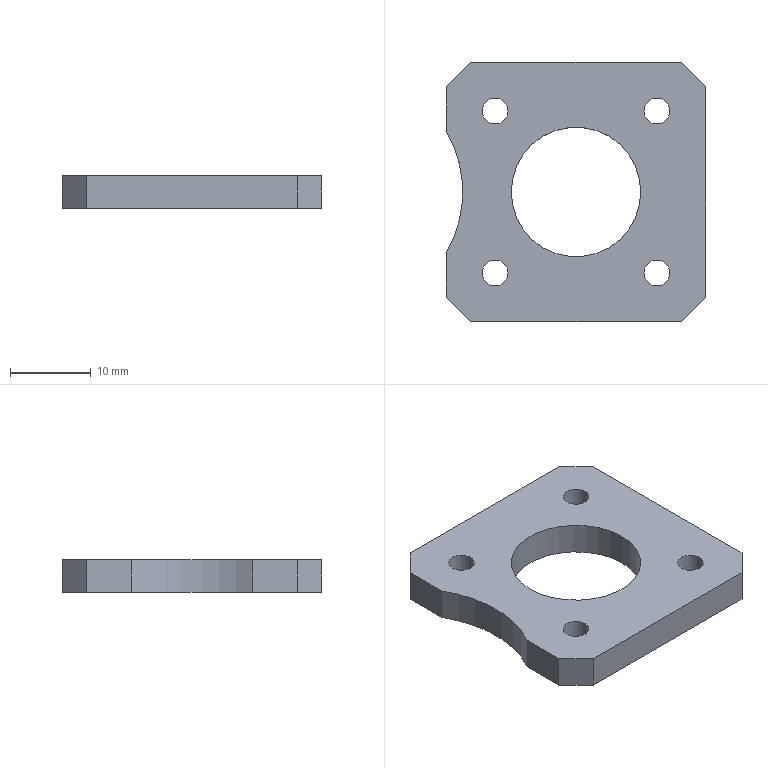Part | SolidWorks | features BaseBody 1 | 1 solid | 22 faces | box 32 x 32 x 4 mm | volume 3010 mm3 | cylinder 11 | plane 11 | commonest cylinder face diameters 3.2 x8 16 x2 30 x1
STEP:
#1=CARTESIAN_POINT('',(-11.6,10.,4.));
#2=VERTEX_POINT('',#1);
#3=CARTESIAN_POINT('',(-8.4,10.,4.));
#4=VERTEX_POINT('',#3);
#5=CARTESIAN_POINT('',(-10.,10.,4.));
#6=DIRECTION('',(0.,0.,1.));
#7=DIRECTION('',(-1.,0.,0.));
#8=AXIS2_PLACEMENT_3D('',#5,#6,#7);
#9=CIRCLE('',#8,1.6);
#10=EDGE_CURVE('',#2,#4,#9,.T.);
#11=ORIENTED_EDGE('',*,*,#10,.T.);
#12=CARTESIAN_POINT('',(-8.4,10.,0.));
#13=VERTEX_POINT('',#12);
#14=CARTESIAN_POINT('',(-8.4,10.,4.));
#15=DIRECTION('',(0.,0.,-1.));
#16=VECTOR('',#15,1000.);
#17=LINE('',#14,#16);
#18=EDGE_CURVE('',#4,#13,#17,.T.);
#19=ORIENTED_EDGE('',*,*,#18,.T.);
#20=CARTESIAN_POINT('',(-11.6,10.,0.));
#21=VERTEX_POINT('',#20);
#22=CARTESIAN_POINT('',(-10.,10.,0.));
#23=DIRECTION('',(0.,0.,-1.));
#24=DIRECTION('',(-1.,0.,0.));
#25=AXIS2_PLACEMENT_3D('',#22,#23,#24);
#26=CIRCLE('',#25,1.6);
#27=EDGE_CURVE('',#13,#21,#26,.T.);
#28=ORIENTED_EDGE('',*,*,#27,.T.);
#29=CARTESIAN_POINT('',(-11.6,10.,4.));
#30=DIRECTION('',(0.,0.,-1.));
#31=VECTOR('',#30,1000.);
#32=LINE('',#29,#31);
#33=EDGE_CURVE('',#2,#21,#32,.T.);
#34=ORIENTED_EDGE('',*,*,#33,.F.);
#35=EDGE_LOOP('',(#11,#19,#28,#34));
#36=FACE_OUTER_BOUND('',#35,.T.);
#37=CARTESIAN_POINT('',(-10.,10.,4.));
#38=DIRECTION('',(0.,0.,-1.));
#39=DIRECTION('',(-1.,0.,0.));
#40=AXIS2_PLACEMENT_3D('',#37,#38,#39);
#41=CYLINDRICAL_SURFACE('',#40,1.6);
#42=ADVANCED_FACE('',(#36),#41,.F.);
#43=CARTESIAN_POINT('',(8.,0.,4.));
#44=VERTEX_POINT('',#43);
#45=CARTESIAN_POINT('',(-8.,0.,4.));
#46=VERTEX_POINT('',#45);
#47=CARTESIAN_POINT('',(0.,0.,4.));
#48=DIRECTION('',(0.,0.,-1.));
#49=DIRECTION('',(-1.,0.,0.));
#50=AXIS2_PLACEMENT_3D('',#47,#48,#49);
#51=CIRCLE('',#50,8.);
#52=EDGE_CURVE('',#44,#46,#51,.T.);
#53=ORIENTED_EDGE('',*,*,#52,.F.);
#54=CARTESIAN_POINT('',(8.,0.,0.));
#55=VERTEX_POINT('',#54);
#56=CARTESIAN_POINT('',(8.,0.,4.));
#57=DIRECTION('',(0.,0.,-1.));
#58=VECTOR('',#57,1000.);
#59=LINE('',#56,#58);
#60=EDGE_CURVE('',#44,#55,#59,.T.);
#61=ORIENTED_EDGE('',*,*,#60,.T.);
#62=CARTESIAN_POINT('',(-8.,0.,0.));
#63=VERTEX_POINT('',#62);
#64=CARTESIAN_POINT('',(0.,0.,0.));
#65=DIRECTION('',(0.,0.,-1.));
#66=DIRECTION('',(-1.,0.,0.));
#67=AXIS2_PLACEMENT_3D('',#64,#65,#66);
#68=CIRCLE('',#67,8.);
#69=EDGE_CURVE('',#55,#63,#68,.T.);
#70=ORIENTED_EDGE('',*,*,#69,.T.);
#71=CARTESIAN_POINT('',(-8.,0.,4.));
#72=DIRECTION('',(0.,0.,-1.));
#73=VECTOR('',#72,1000.);
#74=LINE('',#71,#73);
#75=EDGE_CURVE('',#46,#63,#74,.T.);
#76=ORIENTED_EDGE('',*,*,#75,.F.);
#77=EDGE_LOOP('',(#53,#61,#70,#76));
#78=FACE_OUTER_BOUND('',#77,.T.);
#79=CARTESIAN_POINT('',(0.,0.,4.));
#80=DIRECTION('',(0.,0.,-1.));
#81=DIRECTION('',(-1.,0.,0.));
#82=AXIS2_PLACEMENT_3D('',#79,#80,#81);
#83=CYLINDRICAL_SURFACE('',#82,8.);
#84=ADVANCED_FACE('',(#78),#83,.F.);
#85=CARTESIAN_POINT('',(-8.4,-10.,4.));
#86=VERTEX_POINT('',#85);
#87=CARTESIAN_POINT('',(-11.6,-10.,4.));
#88=VERTEX_POINT('',#87);
#89=CARTESIAN_POINT('',(-10.,-10.,4.));
#90=DIRECTION('',(0.,0.,-1.));
#91=DIRECTION('',(-1.,0.,0.));
#92=AXIS2_PLACEMENT_3D('',#89,#90,#91);
#93=CIRCLE('',#92,1.6);
#94=EDGE_CURVE('',#86,#88,#93,.T.);
#95=ORIENTED_EDGE('',*,*,#94,.F.);
#96=CARTESIAN_POINT('',(-8.4,-10.,0.));
#97=VERTEX_POINT('',#96);
#98=CARTESIAN_POINT('',(-8.4,-10.,4.));
#99=DIRECTION('',(0.,0.,-1.));
#100=VECTOR('',#99,1000.);
#101=LINE('',#98,#100);
#102=EDGE_CURVE('',#86,#97,#101,.T.);
#103=ORIENTED_EDGE('',*,*,#102,.T.);
#104=CARTESIAN_POINT('',(-11.6,-10.,0.));
#105=VERTEX_POINT('',#104);
#106=CARTESIAN_POINT('',(-10.,-10.,0.));
#107=DIRECTION('',(0.,0.,-1.));
#108=DIRECTION('',(-1.,0.,0.));
#109=AXIS2_PLACEMENT_3D('',#106,#107,#108);
#110=CIRCLE('',#109,1.6);
#111=EDGE_CURVE('',#97,#105,#110,.T.);
#112=ORIENTED_EDGE('',*,*,#111,.T.);
#113=CARTESIAN_POINT('',(-11.6,-10.,4.));
#114=DIRECTION('',(0.,0.,-1.));
#115=VECTOR('',#114,1000.);
#116=LINE('',#113,#115);
#117=EDGE_CURVE('',#88,#105,#116,.T.);
#118=ORIENTED_EDGE('',*,*,#117,.F.);
#119=EDGE_LOOP('',(#95,#103,#112,#118));
#120=FACE_OUTER_BOUND('',#119,.T.);
#121=CARTESIAN_POINT('',(-10.,-10.,4.));
#122=DIRECTION('',(0.,0.,-1.));
#123=DIRECTION('',(-1.,0.,0.));
#124=AXIS2_PLACEMENT_3D('',#121,#122,#123);
#125=CYLINDRICAL_SURFACE('',#124,1.6);
#126=ADVANCED_FACE('',(#120),#125,.F.);
#127=CARTESIAN_POINT('',(11.6,-10.,4.));
#128=VERTEX_POINT('',#127);
#129=CARTESIAN_POINT('',(8.4,-10.,4.));
#130=VERTEX_POINT('',#129);
#131=CARTESIAN_POINT('',(10.,-10.,4.));
#132=DIRECTION('',(0.,0.,-1.));
#133=DIRECTION('',(-1.,0.,0.));
#134=AXIS2_PLACEMENT_3D('',#131,#132,#133);
#135=CIRCLE('',#134,1.6);
#136=EDGE_CURVE('',#128,#130,#135,.T.);
#137=ORIENTED_EDGE('',*,*,#136,.F.);
#138=CARTESIAN_POINT('',(11.6,-10.,0.));
#139=VERTEX_POINT('',#138);
#140=CARTESIAN_POINT('',(11.6,-10.,4.));
#141=DIRECTION('',(0.,0.,-1.));
#142=VECTOR('',#141,1000.);
#143=LINE('',#140,#142);
#144=EDGE_CURVE('',#128,#139,#143,.T.);
#145=ORIENTED_EDGE('',*,*,#144,.T.);
#146=CARTESIAN_POINT('',(8.4,-10.,0.));
#147=VERTEX_POINT('',#146);
#148=CARTESIAN_POINT('',(10.,-10.,0.));
#149=DIRECTION('',(0.,0.,-1.));
#150=DIRECTION('',(-1.,0.,0.));
#151=AXIS2_PLACEMENT_3D('',#148,#149,#150);
#152=CIRCLE('',#151,1.6);
#153=EDGE_CURVE('',#139,#147,#152,.T.);
#154=ORIENTED_EDGE('',*,*,#153,.T.);
#155=CARTESIAN_POINT('',(8.4,-10.,4.));
#156=DIRECTION('',(0.,0.,-1.));
#157=VECTOR('',#156,1000.);
#158=LINE('',#155,#157);
#159=EDGE_CURVE('',#130,#147,#158,.T.);
#160=ORIENTED_EDGE('',*,*,#159,.F.);
#161=EDGE_LOOP('',(#137,#145,#154,#160));
#162=FACE_OUTER_BOUND('',#161,.T.);
#163=CARTESIAN_POINT('',(10.,-10.,4.));
#164=DIRECTION('',(0.,0.,-1.));
#165=DIRECTION('',(-1.,0.,0.));
#166=AXIS2_PLACEMENT_3D('',#163,#164,#165);
#167=CYLINDRICAL_SURFACE('',#166,1.6);
#168=ADVANCED_FACE('',(#162),#167,.F.);
#169=CARTESIAN_POINT('',(11.6,10.,4.));
#170=VERTEX_POINT('',#169);
#171=CARTESIAN_POINT('',(8.4,10.,4.));
#172=VERTEX_POINT('',#171);
#173=CARTESIAN_POINT('',(10.,10.,4.));
#174=DIRECTION('',(0.,0.,-1.));
#175=DIRECTION('',(-1.,0.,0.));
#176=AXIS2_PLACEMENT_3D('',#173,#174,#175);
#177=CIRCLE('',#176,1.6);
#178=EDGE_CURVE('',#170,#172,#177,.T.);
#179=ORIENTED_EDGE('',*,*,#178,.F.);
#180=CARTESIAN_POINT('',(11.6,10.,0.));
#181=VERTEX_POINT('',#180);
#182=CARTESIAN_POINT('',(11.6,10.,4.));
#183=DIRECTION('',(0.,0.,-1.));
#184=VECTOR('',#183,1000.);
#185=LINE('',#182,#184);
#186=EDGE_CURVE('',#170,#181,#185,.T.);
#187=ORIENTED_EDGE('',*,*,#186,.T.);
#188=CARTESIAN_POINT('',(8.4,10.,0.));
#189=VERTEX_POINT('',#188);
#190=CARTESIAN_POINT('',(10.,10.,0.));
#191=DIRECTION('',(0.,0.,-1.));
#192=DIRECTION('',(-1.,0.,0.));
#193=AXIS2_PLACEMENT_3D('',#190,#191,#192);
#194=CIRCLE('',#193,1.6);
#195=EDGE_CURVE('',#181,#189,#194,.T.);
#196=ORIENTED_EDGE('',*,*,#195,.T.);
#197=CARTESIAN_POINT('',(8.4,10.,4.));
#198=DIRECTION('',(0.,0.,-1.));
#199=VECTOR('',#198,1000.);
#200=LINE('',#197,#199);
#201=EDGE_CURVE('',#172,#189,#200,.T.);
#202=ORIENTED_EDGE('',*,*,#201,.F.);
#203=EDGE_LOOP('',(#179,#187,#196,#202));
#204=FACE_OUTER_BOUND('',#203,.T.);
#205=CARTESIAN_POINT('',(10.,10.,4.));
#206=DIRECTION('',(0.,0.,-1.));
#207=DIRECTION('',(-1.,0.,0.));
#208=AXIS2_PLACEMENT_3D('',#205,#206,#207);
#209=CYLINDRICAL_SURFACE('',#208,1.6);
#210=ADVANCED_FACE('',(#204),#209,.F.);
#211=ORIENTED_EDGE('',*,*,#18,.F.);
#212=CARTESIAN_POINT('',(-10.,10.,4.));
#213=DIRECTION('',(0.,0.,1.));
#214=DIRECTION('',(-1.,0.,0.));
#215=AXIS2_PLACEMENT_3D('',#212,#213,#214);
#216=CIRCLE('',#215,1.6);
#217=EDGE_CURVE('',#4,#2,#216,.T.);
#218=ORIENTED_EDGE('',*,*,#217,.T.);
#219=ORIENTED_EDGE('',*,*,#33,.T.);
#220=CARTESIAN_POINT('',(-10.,10.,0.));
#221=DIRECTION('',(0.,0.,-1.));
#222=DIRECTION('',(-1.,0.,0.));
#223=AXIS2_PLACEMENT_3D('',#220,#221,#222);
#224=CIRCLE('',#223,1.6);
#225=EDGE_CURVE('',#21,#13,#224,.T.);
#226=ORIENTED_EDGE('',*,*,#225,.T.);
#227=EDGE_LOOP('',(#211,#218,#219,#226));
#228=FACE_OUTER_BOUND('',#227,.T.);
#229=CARTESIAN_POINT('',(-10.,10.,4.));
#230=DIRECTION('',(0.,0.,-1.));
#231=DIRECTION('',(-1.,0.,0.));
#232=AXIS2_PLACEMENT_3D('',#229,#230,#231);
#233=CYLINDRICAL_SURFACE('',#232,1.6);
#234=ADVANCED_FACE('',(#228),#233,.F.);
#235=ORIENTED_EDGE('',*,*,#225,.F.);
#236=ORIENTED_EDGE('',*,*,#27,.F.);
#237=EDGE_LOOP('',(#235,#236));
#238=FACE_BOUND('',#237,.T.);
#239=CARTESIAN_POINT('',(0.,0.,0.));
#240=DIRECTION('',(0.,0.,-1.));
#241=DIRECTION('',(-1.,0.,0.));
#242=AXIS2_PLACEMENT_3D('',#239,#240,#241);
#243=CIRCLE('',#242,8.);
#244=EDGE_CURVE('',#63,#55,#243,.T.);
#245=ORIENTED_EDGE('',*,*,#244,.F.);
#246=ORIENTED_EDGE('',*,*,#69,.F.);
#247=EDGE_LOOP('',(#245,#246));
#248=FACE_BOUND('',#247,.T.);
#249=CARTESIAN_POINT('',(-10.,-10.,0.));
#250=DIRECTION('',(0.,0.,-1.));
#251=DIRECTION('',(-1.,0.,0.));
#252=AXIS2_PLACEMENT_3D('',#249,#250,#251);
#253=CIRCLE('',#252,1.6);
#254=EDGE_CURVE('',#105,#97,#253,.T.);
#255=ORIENTED_EDGE('',*,*,#254,.F.);
#256=ORIENTED_EDGE('',*,*,#111,.F.);
#257=EDGE_LOOP('',(#255,#256));
#258=FACE_BOUND('',#257,.T.);
#259=CARTESIAN_POINT('',(10.,-10.,0.));
#260=DIRECTION('',(0.,0.,-1.));
#261=DIRECTION('',(-1.,0.,0.));
#262=AXIS2_PLACEMENT_3D('',#259,#260,#261);
#263=CIRCLE('',#262,1.6);
#264=EDGE_CURVE('',#147,#139,#263,.T.);
#265=ORIENTED_EDGE('',*,*,#264,.F.);
#266=ORIENTED_EDGE('',*,*,#153,.F.);
#267=EDGE_LOOP('',(#265,#266));
#268=FACE_BOUND('',#267,.T.);
#269=CARTESIAN_POINT('',(10.,10.,0.));
#270=DIRECTION('',(0.,0.,-1.));
#271=DIRECTION('',(-1.,0.,0.));
#272=AXIS2_PLACEMENT_3D('',#269,#270,#271);
#273=CIRCLE('',#272,1.6);
#274=EDGE_CURVE('',#189,#181,#273,.T.);
#275=ORIENTED_EDGE('',*,*,#274,.F.);
#276=ORIENTED_EDGE('',*,*,#195,.F.);
#277=EDGE_LOOP('',(#275,#276));
#278=FACE_BOUND('',#277,.T.);
#279=CARTESIAN_POINT('',(13.,-16.,0.));
#280=VERTEX_POINT('',#279);
#281=CARTESIAN_POINT('',(16.,-13.,0.));
#282=VERTEX_POINT('',#281);
#283=CARTESIAN_POINT('',(16.,-13.,0.));
#284=DIRECTION('',(0.7071,0.7071,0.));
#285=VECTOR('',#284,1000.);
#286=LINE('',#283,#285);
#287=EDGE_CURVE('',#280,#282,#286,.T.);
#288=ORIENTED_EDGE('',*,*,#287,.F.);
#289=CARTESIAN_POINT('',(-13.,-16.,0.));
#290=VERTEX_POINT('',#289);
#291=CARTESIAN_POINT('',(0.,-16.,0.));
#292=DIRECTION('',(1.,0.,0.));
#293=VECTOR('',#292,1000.);
#294=LINE('',#291,#293);
#295=EDGE_CURVE('',#290,#280,#294,.T.);
#296=ORIENTED_EDGE('',*,*,#295,.F.);
#297=CARTESIAN_POINT('',(-16.,-13.,0.));
#298=VERTEX_POINT('',#297);
#299=CARTESIAN_POINT('',(-13.,-16.,0.));
#300=DIRECTION('',(0.7071,-0.7071,0.));
#301=VECTOR('',#300,1000.);
#302=LINE('',#299,#301);
#303=EDGE_CURVE('',#298,#290,#302,.T.);
#304=ORIENTED_EDGE('',*,*,#303,.F.);
#305=CARTESIAN_POINT('',(-16.,-7.483,0.));
#306=VERTEX_POINT('',#305);
#307=CARTESIAN_POINT('',(-16.,0.,0.));
#308=DIRECTION('',(0.,-1.,0.));
#309=VECTOR('',#308,1000.);
#310=LINE('',#307,#309);
#311=EDGE_CURVE('',#306,#298,#310,.T.);
#312=ORIENTED_EDGE('',*,*,#311,.F.);
#313=CARTESIAN_POINT('',(-16.,7.483,0.));
#314=VERTEX_POINT('',#313);
#315=CARTESIAN_POINT('',(-29.,0.,0.));
#316=DIRECTION('',(0.,0.,-1.));
#317=DIRECTION('',(-1.,0.,0.));
#318=AXIS2_PLACEMENT_3D('',#315,#316,#317);
#319=CIRCLE('',#318,15.);
#320=EDGE_CURVE('',#314,#306,#319,.T.);
#321=ORIENTED_EDGE('',*,*,#320,.F.);
#322=CARTESIAN_POINT('',(-16.,13.,0.));
#323=VERTEX_POINT('',#322);
#324=CARTESIAN_POINT('',(-16.,0.,0.));
#325=DIRECTION('',(0.,-1.,0.));
#326=VECTOR('',#325,1000.);
#327=LINE('',#324,#326);
#328=EDGE_CURVE('',#323,#314,#327,.T.);
#329=ORIENTED_EDGE('',*,*,#328,.F.);
#330=CARTESIAN_POINT('',(-13.,16.,0.));
#331=VERTEX_POINT('',#330);
#332=CARTESIAN_POINT('',(-16.,13.,0.));
#333=DIRECTION('',(-0.7071,-0.7071,0.));
#334=VECTOR('',#333,1000.);
#335=LINE('',#332,#334);
#336=EDGE_CURVE('',#331,#323,#335,.T.);
#337=ORIENTED_EDGE('',*,*,#336,.F.);
#338=CARTESIAN_POINT('',(13.,16.,0.));
#339=VERTEX_POINT('',#338);
#340=CARTESIAN_POINT('',(0.,16.,0.));
#341=DIRECTION('',(-1.,0.,0.));
#342=VECTOR('',#341,1000.);
#343=LINE('',#340,#342);
#344=EDGE_CURVE('',#339,#331,#343,.T.);
#345=ORIENTED_EDGE('',*,*,#344,.F.);
#346=CARTESIAN_POINT('',(16.,13.,0.));
#347=VERTEX_POINT('',#346);
#348=CARTESIAN_POINT('',(13.,16.,0.));
#349=DIRECTION('',(-0.7071,0.7071,0.));
#350=VECTOR('',#349,1000.);
#351=LINE('',#348,#350);
#352=EDGE_CURVE('',#347,#339,#351,.T.);
#353=ORIENTED_EDGE('',*,*,#352,.F.);
#354=CARTESIAN_POINT('',(16.,0.,0.));
#355=DIRECTION('',(0.,1.,0.));
#356=VECTOR('',#355,1000.);
#357=LINE('',#354,#356);
#358=EDGE_CURVE('',#282,#347,#357,.T.);
#359=ORIENTED_EDGE('',*,*,#358,.F.);
#360=EDGE_LOOP('',(#288,#296,#304,#312,#321,#329,#337,#345,#353,#359));
#361=FACE_OUTER_BOUND('',#360,.T.);
#362=CARTESIAN_POINT('',(-16.,-16.,0.));
#363=DIRECTION('',(0.,0.,1.));
#364=DIRECTION('',(1.,0.,0.));
#365=AXIS2_PLACEMENT_3D('',#362,#363,#364);
#366=PLANE('',#365);
#367=ADVANCED_FACE('',(#238,#248,#258,#268,#278,#361),#366,.F.);
#368=ORIENTED_EDGE('',*,*,#10,.F.);
#369=ORIENTED_EDGE('',*,*,#217,.F.);
#370=EDGE_LOOP('',(#368,#369));
#371=FACE_BOUND('',#370,.T.);
#372=CARTESIAN_POINT('',(0.,0.,4.));
#373=DIRECTION('',(0.,0.,-1.));
#374=DIRECTION('',(-1.,0.,0.));
#375=AXIS2_PLACEMENT_3D('',#372,#373,#374);
#376=CIRCLE('',#375,8.);
#377=EDGE_CURVE('',#46,#44,#376,.T.);
#378=ORIENTED_EDGE('',*,*,#377,.T.);
#379=ORIENTED_EDGE('',*,*,#52,.T.);
#380=EDGE_LOOP('',(#378,#379));
#381=FACE_BOUND('',#380,.T.);
#382=CARTESIAN_POINT('',(-10.,-10.,4.));
#383=DIRECTION('',(0.,0.,-1.));
#384=DIRECTION('',(-1.,0.,0.));
#385=AXIS2_PLACEMENT_3D('',#382,#383,#384);
#386=CIRCLE('',#385,1.6);
#387=EDGE_CURVE('',#88,#86,#386,.T.);
#388=ORIENTED_EDGE('',*,*,#387,.T.);
#389=ORIENTED_EDGE('',*,*,#94,.T.);
#390=EDGE_LOOP('',(#388,#389));
#391=FACE_BOUND('',#390,.T.);
#392=CARTESIAN_POINT('',(10.,-10.,4.));
#393=DIRECTION('',(0.,0.,-1.));
#394=DIRECTION('',(-1.,0.,0.));
#395=AXIS2_PLACEMENT_3D('',#392,#393,#394);
#396=CIRCLE('',#395,1.6);
#397=EDGE_CURVE('',#130,#128,#396,.T.);
#398=ORIENTED_EDGE('',*,*,#397,.T.);
#399=ORIENTED_EDGE('',*,*,#136,.T.);
#400=EDGE_LOOP('',(#398,#399));
#401=FACE_BOUND('',#400,.T.);
#402=CARTESIAN_POINT('',(10.,10.,4.));
#403=DIRECTION('',(0.,0.,-1.));
#404=DIRECTION('',(-1.,0.,0.));
#405=AXIS2_PLACEMENT_3D('',#402,#403,#404);
#406=CIRCLE('',#405,1.6);
#407=EDGE_CURVE('',#172,#170,#406,.T.);
#408=ORIENTED_EDGE('',*,*,#407,.T.);
#409=ORIENTED_EDGE('',*,*,#178,.T.);
#410=EDGE_LOOP('',(#408,#409));
#411=FACE_BOUND('',#410,.T.);
#412=CARTESIAN_POINT('',(-13.,-16.,4.));
#413=VERTEX_POINT('',#412);
#414=CARTESIAN_POINT('',(13.,-16.,4.));
#415=VERTEX_POINT('',#414);
#416=CARTESIAN_POINT('',(0.,-16.,4.));
#417=DIRECTION('',(1.,0.,0.));
#418=VECTOR('',#417,1000.);
#419=LINE('',#416,#418);
#420=EDGE_CURVE('',#413,#415,#419,.T.);
#421=ORIENTED_EDGE('',*,*,#420,.T.);
#422=CARTESIAN_POINT('',(16.,-13.,4.));
#423=VERTEX_POINT('',#422);
#424=CARTESIAN_POINT('',(13.,-16.,4.));
#425=DIRECTION('',(0.7071,0.7071,0.));
#426=VECTOR('',#425,1000.);
#427=LINE('',#424,#426);
#428=EDGE_CURVE('',#415,#423,#427,.T.);
#429=ORIENTED_EDGE('',*,*,#428,.T.);
#430=CARTESIAN_POINT('',(16.,13.,4.));
#431=VERTEX_POINT('',#430);
#432=CARTESIAN_POINT('',(16.,0.,4.));
#433=DIRECTION('',(0.,1.,0.));
#434=VECTOR('',#433,1000.);
#435=LINE('',#432,#434);
#436=EDGE_CURVE('',#423,#431,#435,.T.);
#437=ORIENTED_EDGE('',*,*,#436,.T.);
#438=CARTESIAN_POINT('',(13.,16.,4.));
#439=VERTEX_POINT('',#438);
#440=CARTESIAN_POINT('',(16.,13.,4.));
#441=DIRECTION('',(-0.7071,0.7071,0.));
#442=VECTOR('',#441,1000.);
#443=LINE('',#440,#442);
#444=EDGE_CURVE('',#431,#439,#443,.T.);
#445=ORIENTED_EDGE('',*,*,#444,.T.);
#446=CARTESIAN_POINT('',(-13.,16.,4.));
#447=VERTEX_POINT('',#446);
#448=CARTESIAN_POINT('',(0.,16.,4.));
#449=DIRECTION('',(-1.,0.,0.));
#450=VECTOR('',#449,1000.);
#451=LINE('',#448,#450);
#452=EDGE_CURVE('',#439,#447,#451,.T.);
#453=ORIENTED_EDGE('',*,*,#452,.T.);
#454=CARTESIAN_POINT('',(-16.,13.,4.));
#455=VERTEX_POINT('',#454);
#456=CARTESIAN_POINT('',(-13.,16.,4.));
#457=DIRECTION('',(-0.7071,-0.7071,0.));
#458=VECTOR('',#457,1000.);
#459=LINE('',#456,#458);
#460=EDGE_CURVE('',#447,#455,#459,.T.);
#461=ORIENTED_EDGE('',*,*,#460,.T.);
#462=CARTESIAN_POINT('',(-16.,7.483,4.));
#463=VERTEX_POINT('',#462);
#464=CARTESIAN_POINT('',(-16.,0.,4.));
#465=DIRECTION('',(0.,-1.,0.));
#466=VECTOR('',#465,1000.);
#467=LINE('',#464,#466);
#468=EDGE_CURVE('',#455,#463,#467,.T.);
#469=ORIENTED_EDGE('',*,*,#468,.T.);
#470=CARTESIAN_POINT('',(-16.,-7.483,4.));
#471=VERTEX_POINT('',#470);
#472=CARTESIAN_POINT('',(-29.,0.,4.));
#473=DIRECTION('',(0.,0.,-1.));
#474=DIRECTION('',(-1.,0.,0.));
#475=AXIS2_PLACEMENT_3D('',#472,#473,#474);
#476=CIRCLE('',#475,15.);
#477=EDGE_CURVE('',#463,#471,#476,.T.);
#478=ORIENTED_EDGE('',*,*,#477,.T.);
#479=CARTESIAN_POINT('',(-16.,-13.,4.));
#480=VERTEX_POINT('',#479);
#481=CARTESIAN_POINT('',(-16.,0.,4.));
#482=DIRECTION('',(0.,-1.,0.));
#483=VECTOR('',#482,1000.);
#484=LINE('',#481,#483);
#485=EDGE_CURVE('',#471,#480,#484,.T.);
#486=ORIENTED_EDGE('',*,*,#485,.T.);
#487=CARTESIAN_POINT('',(-16.,-13.,4.));
#488=DIRECTION('',(0.7071,-0.7071,0.));
#489=VECTOR('',#488,1000.);
#490=LINE('',#487,#489);
#491=EDGE_CURVE('',#480,#413,#490,.T.);
#492=ORIENTED_EDGE('',*,*,#491,.T.);
#493=EDGE_LOOP('',(#421,#429,#437,#445,#453,#461,#469,#478,#486,#492));
#494=FACE_OUTER_BOUND('',#493,.T.);
#495=CARTESIAN_POINT('',(-16.,-16.,4.));
#496=DIRECTION('',(0.,0.,1.));
#497=DIRECTION('',(1.,0.,0.));
#498=AXIS2_PLACEMENT_3D('',#495,#496,#497);
#499=PLANE('',#498);
#500=ADVANCED_FACE('',(#371,#381,#391,#401,#411,#494),#499,.T.);
#501=ORIENTED_EDGE('',*,*,#60,.F.);
#502=ORIENTED_EDGE('',*,*,#377,.F.);
#503=ORIENTED_EDGE('',*,*,#75,.T.);
#504=ORIENTED_EDGE('',*,*,#244,.T.);
#505=EDGE_LOOP('',(#501,#502,#503,#504));
#506=FACE_OUTER_BOUND('',#505,.T.);
#507=CARTESIAN_POINT('',(0.,0.,4.));
#508=DIRECTION('',(0.,0.,-1.));
#509=DIRECTION('',(-1.,0.,0.));
#510=AXIS2_PLACEMENT_3D('',#507,#508,#509);
#511=CYLINDRICAL_SURFACE('',#510,8.);
#512=ADVANCED_FACE('',(#506),#511,.F.);
#513=ORIENTED_EDGE('',*,*,#102,.F.);
#514=ORIENTED_EDGE('',*,*,#387,.F.);
#515=ORIENTED_EDGE('',*,*,#117,.T.);
#516=ORIENTED_EDGE('',*,*,#254,.T.);
#517=EDGE_LOOP('',(#513,#514,#515,#516));
#518=FACE_OUTER_BOUND('',#517,.T.);
#519=CARTESIAN_POINT('',(-10.,-10.,4.));
#520=DIRECTION('',(0.,0.,-1.));
#521=DIRECTION('',(-1.,0.,0.));
#522=AXIS2_PLACEMENT_3D('',#519,#520,#521);
#523=CYLINDRICAL_SURFACE('',#522,1.6);
#524=ADVANCED_FACE('',(#518),#523,.F.);
#525=ORIENTED_EDGE('',*,*,#144,.F.);
#526=ORIENTED_EDGE('',*,*,#397,.F.);
#527=ORIENTED_EDGE('',*,*,#159,.T.);
#528=ORIENTED_EDGE('',*,*,#264,.T.);
#529=EDGE_LOOP('',(#525,#526,#527,#528));
#530=FACE_OUTER_BOUND('',#529,.T.);
#531=CARTESIAN_POINT('',(10.,-10.,4.));
#532=DIRECTION('',(0.,0.,-1.));
#533=DIRECTION('',(-1.,0.,0.));
#534=AXIS2_PLACEMENT_3D('',#531,#532,#533);
#535=CYLINDRICAL_SURFACE('',#534,1.6);
#536=ADVANCED_FACE('',(#530),#535,.F.);
#537=ORIENTED_EDGE('',*,*,#186,.F.);
#538=ORIENTED_EDGE('',*,*,#407,.F.);
#539=ORIENTED_EDGE('',*,*,#201,.T.);
#540=ORIENTED_EDGE('',*,*,#274,.T.);
#541=EDGE_LOOP('',(#537,#538,#539,#540));
#542=FACE_OUTER_BOUND('',#541,.T.);
#543=CARTESIAN_POINT('',(10.,10.,4.));
#544=DIRECTION('',(0.,0.,-1.));
#545=DIRECTION('',(-1.,0.,0.));
#546=AXIS2_PLACEMENT_3D('',#543,#544,#545);
#547=CYLINDRICAL_SURFACE('',#546,1.6);
#548=ADVANCED_FACE('',(#542),#547,.F.);
#549=CARTESIAN_POINT('',(16.,13.,2.));
#550=DIRECTION('',(0.,0.,-1.));
#551=VECTOR('',#550,1000.);
#552=LINE('',#549,#551);
#553=EDGE_CURVE('',#431,#347,#552,.T.);
#554=ORIENTED_EDGE('',*,*,#553,.F.);
#555=ORIENTED_EDGE('',*,*,#436,.F.);
#556=CARTESIAN_POINT('',(16.,-13.,2.));
#557=DIRECTION('',(0.,0.,1.));
#558=VECTOR('',#557,1000.);
#559=LINE('',#556,#558);
#560=EDGE_CURVE('',#282,#423,#559,.T.);
#561=ORIENTED_EDGE('',*,*,#560,.F.);
#562=ORIENTED_EDGE('',*,*,#358,.T.);
#563=EDGE_LOOP('',(#554,#555,#561,#562));
#564=FACE_OUTER_BOUND('',#563,.T.);
#565=CARTESIAN_POINT('',(16.,-13.,0.));
#566=DIRECTION('',(-1.,0.,0.));
#567=DIRECTION('',(0.,0.,1.));
#568=AXIS2_PLACEMENT_3D('',#565,#566,#567);
#569=PLANE('',#568);
#570=ADVANCED_FACE('',(#564),#569,.F.);
#571=ORIENTED_EDGE('',*,*,#560,.T.);
#572=ORIENTED_EDGE('',*,*,#428,.F.);
#573=CARTESIAN_POINT('',(13.,-16.,2.));
#574=DIRECTION('',(0.,0.,1.));
#575=VECTOR('',#574,1000.);
#576=LINE('',#573,#575);
#577=EDGE_CURVE('',#280,#415,#576,.T.);
#578=ORIENTED_EDGE('',*,*,#577,.F.);
#579=ORIENTED_EDGE('',*,*,#287,.T.);
#580=EDGE_LOOP('',(#571,#572,#578,#579));
#581=FACE_OUTER_BOUND('',#580,.T.);
#582=CARTESIAN_POINT('',(16.,-13.,0.));
#583=DIRECTION('',(-0.7071,0.7071,0.));
#584=DIRECTION('',(-0.7071,-0.7071,0.));
#585=AXIS2_PLACEMENT_3D('',#582,#583,#584);
#586=PLANE('',#585);
#587=ADVANCED_FACE('',(#581),#586,.F.);
#588=ORIENTED_EDGE('',*,*,#577,.T.);
#589=ORIENTED_EDGE('',*,*,#420,.F.);
#590=CARTESIAN_POINT('',(-13.,-16.,2.));
#591=DIRECTION('',(0.,0.,1.));
#592=VECTOR('',#591,1000.);
#593=LINE('',#590,#592);
#594=EDGE_CURVE('',#290,#413,#593,.T.);
#595=ORIENTED_EDGE('',*,*,#594,.F.);
#596=ORIENTED_EDGE('',*,*,#295,.T.);
#597=EDGE_LOOP('',(#588,#589,#595,#596));
#598=FACE_OUTER_BOUND('',#597,.T.);
#599=CARTESIAN_POINT('',(13.,-16.,0.));
#600=DIRECTION('',(0.,1.,0.));
#601=DIRECTION('',(-1.,0.,0.));
#602=AXIS2_PLACEMENT_3D('',#599,#600,#601);
#603=PLANE('',#602);
#604=ADVANCED_FACE('',(#598),#603,.F.);
#605=ORIENTED_EDGE('',*,*,#594,.T.);
#606=ORIENTED_EDGE('',*,*,#491,.F.);
#607=CARTESIAN_POINT('',(-16.,-13.,2.));
#608=DIRECTION('',(0.,0.,1.));
#609=VECTOR('',#608,1000.);
#610=LINE('',#607,#609);
#611=EDGE_CURVE('',#298,#480,#610,.T.);
#612=ORIENTED_EDGE('',*,*,#611,.F.);
#613=ORIENTED_EDGE('',*,*,#303,.T.);
#614=EDGE_LOOP('',(#605,#606,#612,#613));
#615=FACE_OUTER_BOUND('',#614,.T.);
#616=CARTESIAN_POINT('',(-13.,-16.,0.));
#617=DIRECTION('',(0.7071,0.7071,0.));
#618=DIRECTION('',(-0.7071,0.7071,0.));
#619=AXIS2_PLACEMENT_3D('',#616,#617,#618);
#620=PLANE('',#619);
#621=ADVANCED_FACE('',(#615),#620,.F.);
#622=ORIENTED_EDGE('',*,*,#611,.T.);
#623=ORIENTED_EDGE('',*,*,#485,.F.);
#624=CARTESIAN_POINT('',(-16.,-7.483,2.));
#625=DIRECTION('',(0.,0.,1.));
#626=VECTOR('',#625,1000.);
#627=LINE('',#624,#626);
#628=EDGE_CURVE('',#306,#471,#627,.T.);
#629=ORIENTED_EDGE('',*,*,#628,.F.);
#630=ORIENTED_EDGE('',*,*,#311,.T.);
#631=EDGE_LOOP('',(#622,#623,#629,#630));
#632=FACE_OUTER_BOUND('',#631,.T.);
#633=CARTESIAN_POINT('',(-16.,-13.,0.));
#634=DIRECTION('',(1.,0.,0.));
#635=DIRECTION('',(0.,1.,0.));
#636=AXIS2_PLACEMENT_3D('',#633,#634,#635);
#637=PLANE('',#636);
#638=ADVANCED_FACE('',(#632),#637,.F.);
#639=ORIENTED_EDGE('',*,*,#477,.F.);
#640=CARTESIAN_POINT('',(-16.,7.483,2.));
#641=DIRECTION('',(0.,0.,-1.));
#642=VECTOR('',#641,1000.);
#643=LINE('',#640,#642);
#644=EDGE_CURVE('',#463,#314,#643,.T.);
#645=ORIENTED_EDGE('',*,*,#644,.T.);
#646=ORIENTED_EDGE('',*,*,#320,.T.);
#647=ORIENTED_EDGE('',*,*,#628,.T.);
#648=EDGE_LOOP('',(#639,#645,#646,#647));
#649=FACE_OUTER_BOUND('',#648,.T.);
#650=CARTESIAN_POINT('',(-29.,0.,4.));
#651=DIRECTION('',(0.,0.,-1.));
#652=DIRECTION('',(-1.,0.,0.));
#653=AXIS2_PLACEMENT_3D('',#650,#651,#652);
#654=CYLINDRICAL_SURFACE('',#653,15.);
#655=ADVANCED_FACE('',(#649),#654,.F.);
#656=ORIENTED_EDGE('',*,*,#644,.F.);
#657=ORIENTED_EDGE('',*,*,#468,.F.);
#658=CARTESIAN_POINT('',(-16.,13.,2.));
#659=DIRECTION('',(0.,0.,1.));
#660=VECTOR('',#659,1000.);
#661=LINE('',#658,#660);
#662=EDGE_CURVE('',#323,#455,#661,.T.);
#663=ORIENTED_EDGE('',*,*,#662,.F.);
#664=ORIENTED_EDGE('',*,*,#328,.T.);
#665=EDGE_LOOP('',(#656,#657,#663,#664));
#666=FACE_OUTER_BOUND('',#665,.T.);
#667=CARTESIAN_POINT('',(-16.,7.483,4.));
#668=DIRECTION('',(1.,0.,0.));
#669=DIRECTION('',(0.,0.,-1.));
#670=AXIS2_PLACEMENT_3D('',#667,#668,#669);
#671=PLANE('',#670);
#672=ADVANCED_FACE('',(#666),#671,.F.);
#673=ORIENTED_EDGE('',*,*,#662,.T.);
#674=ORIENTED_EDGE('',*,*,#460,.F.);
#675=CARTESIAN_POINT('',(-13.,16.,2.));
#676=DIRECTION('',(0.,0.,1.));
#677=VECTOR('',#676,1000.);
#678=LINE('',#675,#677);
#679=EDGE_CURVE('',#331,#447,#678,.T.);
#680=ORIENTED_EDGE('',*,*,#679,.F.);
#681=ORIENTED_EDGE('',*,*,#336,.T.);
#682=EDGE_LOOP('',(#673,#674,#680,#681));
#683=FACE_OUTER_BOUND('',#682,.T.);
#684=CARTESIAN_POINT('',(-16.,13.,0.));
#685=DIRECTION('',(0.7071,-0.7071,0.));
#686=DIRECTION('',(0.7071,0.7071,0.));
#687=AXIS2_PLACEMENT_3D('',#684,#685,#686);
#688=PLANE('',#687);
#689=ADVANCED_FACE('',(#683),#688,.F.);
#690=ORIENTED_EDGE('',*,*,#679,.T.);
#691=ORIENTED_EDGE('',*,*,#452,.F.);
#692=CARTESIAN_POINT('',(13.,16.,2.));
#693=DIRECTION('',(0.,0.,1.));
#694=VECTOR('',#693,1000.);
#695=LINE('',#692,#694);
#696=EDGE_CURVE('',#339,#439,#695,.T.);
#697=ORIENTED_EDGE('',*,*,#696,.F.);
#698=ORIENTED_EDGE('',*,*,#344,.T.);
#699=EDGE_LOOP('',(#690,#691,#697,#698));
#700=FACE_OUTER_BOUND('',#699,.T.);
#701=CARTESIAN_POINT('',(-13.,16.,0.));
#702=DIRECTION('',(0.,-1.,0.));
#703=DIRECTION('',(1.,0.,0.));
#704=AXIS2_PLACEMENT_3D('',#701,#702,#703);
#705=PLANE('',#704);
#706=ADVANCED_FACE('',(#700),#705,.F.);
#707=ORIENTED_EDGE('',*,*,#696,.T.);
#708=ORIENTED_EDGE('',*,*,#444,.F.);
#709=ORIENTED_EDGE('',*,*,#553,.T.);
#710=ORIENTED_EDGE('',*,*,#352,.T.);
#711=EDGE_LOOP('',(#707,#708,#709,#710));
#712=FACE_OUTER_BOUND('',#711,.T.);
#713=CARTESIAN_POINT('',(13.,16.,0.));
#714=DIRECTION('',(-0.7071,-0.7071,0.));
#715=DIRECTION('',(0.7071,-0.7071,0.));
#716=AXIS2_PLACEMENT_3D('',#713,#714,#715);
#717=PLANE('',#716);
#718=ADVANCED_FACE('',(#712),#717,.F.);
#719=CLOSED_SHELL('',(#42,#84,#126,#168,#210,#234,#367,#500,#512,#524,#536,#548,#570,#587,#604,#621,#638,#655,#672,#689,#706,#718));
#720=MANIFOLD_SOLID_BREP('',#719);
#721=CARTESIAN_POINT('',(0.,0.,0.));
#722=DIRECTION('',(0.,0.,1.));
#723=DIRECTION('',(1.,0.,0.));
#724=AXIS2_PLACEMENT_3D('',#721,#722,#723);
#725=(LENGTH_UNIT()NAMED_UNIT(*)SI_UNIT(.MILLI.,.METRE.));
#726=UNCERTAINTY_MEASURE_WITH_UNIT(LENGTH_MEASURE(0.00001),#725,'','');
#727=(NAMED_UNIT(*)PLANE_ANGLE_UNIT()SI_UNIT($,.RADIAN.));
#728=(NAMED_UNIT(*)SI_UNIT($,.STERADIAN.)SOLID_ANGLE_UNIT());
#729=(GEOMETRIC_REPRESENTATION_CONTEXT(3)GLOBAL_UNCERTAINTY_ASSIGNED_CONTEXT((#726))GLOBAL_UNIT_ASSIGNED_CONTEXT((#725,#727,#728))REPRESENTATION_CONTEXT('',''));
#730=ADVANCED_BREP_SHAPE_REPRESENTATION('',(#720,#724),#729);